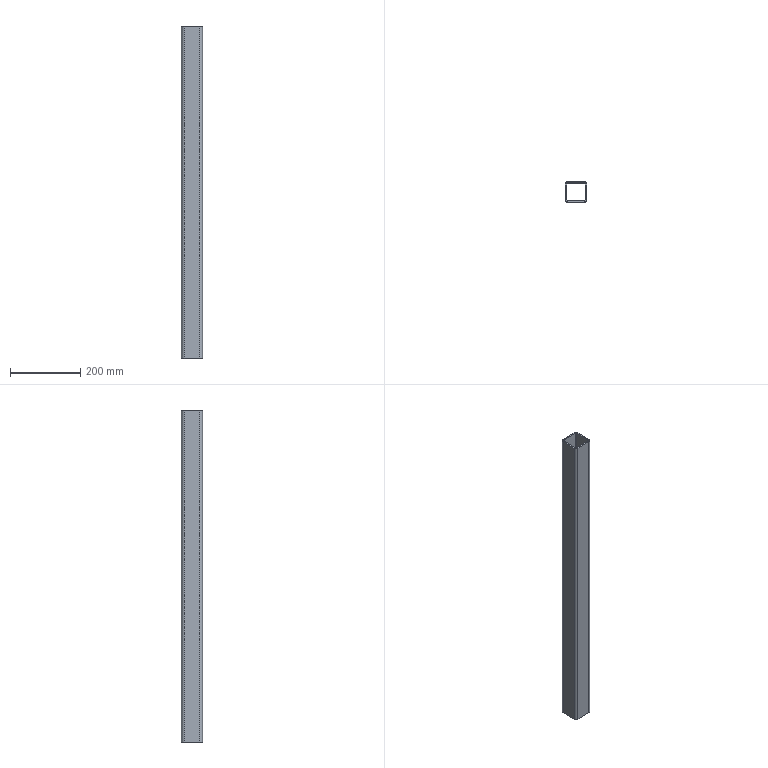Part | SolidWorks | features ICE 1, LibraryFeature 1 | 1 solid | 18 faces | box 60 x 60 x 945 mm | volume 807783 mm3 | plane 10 | cylinder 8 | commonest cylinder face diameters 8 x4 16 x4
STEP:
#1=CARTESIAN_POINT('',(22.,30.,0.));
#2=VERTEX_POINT('',#1);
#3=CARTESIAN_POINT('',(-22.,30.,0.));
#4=VERTEX_POINT('',#3);
#5=CARTESIAN_POINT('',(0.,30.,0.));
#6=DIRECTION('',(-1.,0.,0.));
#7=VECTOR('',#6,1000.);
#8=LINE('',#5,#7);
#9=EDGE_CURVE('',#2,#4,#8,.T.);
#10=ORIENTED_EDGE('',*,*,#9,.T.);
#11=CARTESIAN_POINT('',(-22.,30.,945.));
#12=VERTEX_POINT('',#11);
#13=CARTESIAN_POINT('',(-22.,30.,945.));
#14=DIRECTION('',(0.,0.,-1.));
#15=VECTOR('',#14,1000.);
#16=LINE('',#13,#15);
#17=EDGE_CURVE('',#12,#4,#16,.T.);
#18=ORIENTED_EDGE('',*,*,#17,.F.);
#19=CARTESIAN_POINT('',(22.,30.,945.));
#20=VERTEX_POINT('',#19);
#21=CARTESIAN_POINT('',(0.,30.,945.));
#22=DIRECTION('',(-1.,0.,0.));
#23=VECTOR('',#22,1000.);
#24=LINE('',#21,#23);
#25=EDGE_CURVE('',#20,#12,#24,.T.);
#26=ORIENTED_EDGE('',*,*,#25,.F.);
#27=CARTESIAN_POINT('',(22.,30.,945.));
#28=DIRECTION('',(0.,0.,-1.));
#29=VECTOR('',#28,1000.);
#30=LINE('',#27,#29);
#31=EDGE_CURVE('',#20,#2,#30,.T.);
#32=ORIENTED_EDGE('',*,*,#31,.T.);
#33=EDGE_LOOP('',(#10,#18,#26,#32));
#34=FACE_OUTER_BOUND('',#33,.T.);
#35=CARTESIAN_POINT('',(0.,30.,945.));
#36=DIRECTION('',(0.,-1.,0.));
#37=DIRECTION('',(0.,0.,-1.));
#38=AXIS2_PLACEMENT_3D('',#35,#36,#37);
#39=PLANE('',#38);
#40=ADVANCED_FACE('',(#34),#39,.F.);
#41=CARTESIAN_POINT('',(-30.,22.,0.));
#42=VERTEX_POINT('',#41);
#43=CARTESIAN_POINT('',(-22.,22.,0.));
#44=DIRECTION('',(0.,0.,1.));
#45=DIRECTION('',(1.,0.,0.));
#46=AXIS2_PLACEMENT_3D('',#43,#44,#45);
#47=CIRCLE('',#46,8.);
#48=EDGE_CURVE('',#4,#42,#47,.T.);
#49=ORIENTED_EDGE('',*,*,#48,.T.);
#50=CARTESIAN_POINT('',(-30.,22.,945.));
#51=VERTEX_POINT('',#50);
#52=CARTESIAN_POINT('',(-30.,22.,945.));
#53=DIRECTION('',(0.,0.,-1.));
#54=VECTOR('',#53,1000.);
#55=LINE('',#52,#54);
#56=EDGE_CURVE('',#51,#42,#55,.T.);
#57=ORIENTED_EDGE('',*,*,#56,.F.);
#58=CARTESIAN_POINT('',(-22.,22.,945.));
#59=DIRECTION('',(0.,0.,1.));
#60=DIRECTION('',(1.,0.,0.));
#61=AXIS2_PLACEMENT_3D('',#58,#59,#60);
#62=CIRCLE('',#61,8.);
#63=EDGE_CURVE('',#12,#51,#62,.T.);
#64=ORIENTED_EDGE('',*,*,#63,.F.);
#65=ORIENTED_EDGE('',*,*,#17,.T.);
#66=EDGE_LOOP('',(#49,#57,#64,#65));
#67=FACE_OUTER_BOUND('',#66,.T.);
#68=CARTESIAN_POINT('',(-22.,22.,945.));
#69=DIRECTION('',(0.,0.,-1.));
#70=DIRECTION('',(-1.,0.,0.));
#71=AXIS2_PLACEMENT_3D('',#68,#69,#70);
#72=CYLINDRICAL_SURFACE('',#71,8.);
#73=ADVANCED_FACE('',(#67),#72,.T.);
#74=CARTESIAN_POINT('',(-30.,-22.,0.));
#75=VERTEX_POINT('',#74);
#76=CARTESIAN_POINT('',(-30.,0.,0.));
#77=DIRECTION('',(0.,1.,0.));
#78=VECTOR('',#77,1000.);
#79=LINE('',#76,#78);
#80=EDGE_CURVE('',#75,#42,#79,.T.);
#81=ORIENTED_EDGE('',*,*,#80,.F.);
#82=CARTESIAN_POINT('',(-30.,-22.,945.));
#83=VERTEX_POINT('',#82);
#84=CARTESIAN_POINT('',(-30.,-22.,945.));
#85=DIRECTION('',(0.,0.,-1.));
#86=VECTOR('',#85,1000.);
#87=LINE('',#84,#86);
#88=EDGE_CURVE('',#83,#75,#87,.T.);
#89=ORIENTED_EDGE('',*,*,#88,.F.);
#90=CARTESIAN_POINT('',(-30.,0.,945.));
#91=DIRECTION('',(0.,1.,0.));
#92=VECTOR('',#91,1000.);
#93=LINE('',#90,#92);
#94=EDGE_CURVE('',#83,#51,#93,.T.);
#95=ORIENTED_EDGE('',*,*,#94,.T.);
#96=ORIENTED_EDGE('',*,*,#56,.T.);
#97=EDGE_LOOP('',(#81,#89,#95,#96));
#98=FACE_OUTER_BOUND('',#97,.T.);
#99=CARTESIAN_POINT('',(-30.,0.,945.));
#100=DIRECTION('',(-1.,0.,0.));
#101=DIRECTION('',(0.,0.,1.));
#102=AXIS2_PLACEMENT_3D('',#99,#100,#101);
#103=PLANE('',#102);
#104=ADVANCED_FACE('',(#98),#103,.T.);
#105=CARTESIAN_POINT('',(-22.,-30.,0.));
#106=VERTEX_POINT('',#105);
#107=CARTESIAN_POINT('',(-22.,-22.,0.));
#108=DIRECTION('',(0.,0.,1.));
#109=DIRECTION('',(1.,0.,0.));
#110=AXIS2_PLACEMENT_3D('',#107,#108,#109);
#111=CIRCLE('',#110,8.);
#112=EDGE_CURVE('',#75,#106,#111,.T.);
#113=ORIENTED_EDGE('',*,*,#112,.T.);
#114=CARTESIAN_POINT('',(-22.,-30.,945.));
#115=VERTEX_POINT('',#114);
#116=CARTESIAN_POINT('',(-22.,-30.,945.));
#117=DIRECTION('',(0.,0.,-1.));
#118=VECTOR('',#117,1000.);
#119=LINE('',#116,#118);
#120=EDGE_CURVE('',#115,#106,#119,.T.);
#121=ORIENTED_EDGE('',*,*,#120,.F.);
#122=CARTESIAN_POINT('',(-22.,-22.,945.));
#123=DIRECTION('',(0.,0.,1.));
#124=DIRECTION('',(1.,0.,0.));
#125=AXIS2_PLACEMENT_3D('',#122,#123,#124);
#126=CIRCLE('',#125,8.);
#127=EDGE_CURVE('',#83,#115,#126,.T.);
#128=ORIENTED_EDGE('',*,*,#127,.F.);
#129=ORIENTED_EDGE('',*,*,#88,.T.);
#130=EDGE_LOOP('',(#113,#121,#128,#129));
#131=FACE_OUTER_BOUND('',#130,.T.);
#132=CARTESIAN_POINT('',(-22.,-22.,945.));
#133=DIRECTION('',(0.,0.,-1.));
#134=DIRECTION('',(-1.,0.,0.));
#135=AXIS2_PLACEMENT_3D('',#132,#133,#134);
#136=CYLINDRICAL_SURFACE('',#135,8.);
#137=ADVANCED_FACE('',(#131),#136,.T.);
#138=CARTESIAN_POINT('',(22.,-30.,0.));
#139=VERTEX_POINT('',#138);
#140=CARTESIAN_POINT('',(0.,-30.,0.));
#141=DIRECTION('',(1.,0.,0.));
#142=VECTOR('',#141,1000.);
#143=LINE('',#140,#142);
#144=EDGE_CURVE('',#106,#139,#143,.T.);
#145=ORIENTED_EDGE('',*,*,#144,.T.);
#146=CARTESIAN_POINT('',(22.,-30.,945.));
#147=VERTEX_POINT('',#146);
#148=CARTESIAN_POINT('',(22.,-30.,945.));
#149=DIRECTION('',(0.,0.,-1.));
#150=VECTOR('',#149,1000.);
#151=LINE('',#148,#150);
#152=EDGE_CURVE('',#147,#139,#151,.T.);
#153=ORIENTED_EDGE('',*,*,#152,.F.);
#154=CARTESIAN_POINT('',(0.,-30.,945.));
#155=DIRECTION('',(1.,0.,0.));
#156=VECTOR('',#155,1000.);
#157=LINE('',#154,#156);
#158=EDGE_CURVE('',#115,#147,#157,.T.);
#159=ORIENTED_EDGE('',*,*,#158,.F.);
#160=ORIENTED_EDGE('',*,*,#120,.T.);
#161=EDGE_LOOP('',(#145,#153,#159,#160));
#162=FACE_OUTER_BOUND('',#161,.T.);
#163=CARTESIAN_POINT('',(0.,-30.,945.));
#164=DIRECTION('',(0.,1.,0.));
#165=DIRECTION('',(0.,0.,1.));
#166=AXIS2_PLACEMENT_3D('',#163,#164,#165);
#167=PLANE('',#166);
#168=ADVANCED_FACE('',(#162),#167,.F.);
#169=CARTESIAN_POINT('',(30.,-22.,0.));
#170=VERTEX_POINT('',#169);
#171=CARTESIAN_POINT('',(22.,-22.,0.));
#172=DIRECTION('',(0.,0.,1.));
#173=DIRECTION('',(1.,0.,0.));
#174=AXIS2_PLACEMENT_3D('',#171,#172,#173);
#175=CIRCLE('',#174,8.);
#176=EDGE_CURVE('',#139,#170,#175,.T.);
#177=ORIENTED_EDGE('',*,*,#176,.T.);
#178=CARTESIAN_POINT('',(30.,-22.,945.));
#179=VERTEX_POINT('',#178);
#180=CARTESIAN_POINT('',(30.,-22.,945.));
#181=DIRECTION('',(0.,0.,-1.));
#182=VECTOR('',#181,1000.);
#183=LINE('',#180,#182);
#184=EDGE_CURVE('',#179,#170,#183,.T.);
#185=ORIENTED_EDGE('',*,*,#184,.F.);
#186=CARTESIAN_POINT('',(22.,-22.,945.));
#187=DIRECTION('',(0.,0.,1.));
#188=DIRECTION('',(1.,0.,0.));
#189=AXIS2_PLACEMENT_3D('',#186,#187,#188);
#190=CIRCLE('',#189,8.);
#191=EDGE_CURVE('',#147,#179,#190,.T.);
#192=ORIENTED_EDGE('',*,*,#191,.F.);
#193=ORIENTED_EDGE('',*,*,#152,.T.);
#194=EDGE_LOOP('',(#177,#185,#192,#193));
#195=FACE_OUTER_BOUND('',#194,.T.);
#196=CARTESIAN_POINT('',(22.,-22.,945.));
#197=DIRECTION('',(0.,0.,-1.));
#198=DIRECTION('',(-1.,0.,0.));
#199=AXIS2_PLACEMENT_3D('',#196,#197,#198);
#200=CYLINDRICAL_SURFACE('',#199,8.);
#201=ADVANCED_FACE('',(#195),#200,.T.);
#202=CARTESIAN_POINT('',(30.,22.,0.));
#203=VERTEX_POINT('',#202);
#204=CARTESIAN_POINT('',(30.,0.,0.));
#205=DIRECTION('',(0.,-1.,0.));
#206=VECTOR('',#205,1000.);
#207=LINE('',#204,#206);
#208=EDGE_CURVE('',#203,#170,#207,.T.);
#209=ORIENTED_EDGE('',*,*,#208,.F.);
#210=CARTESIAN_POINT('',(30.,22.,945.));
#211=VERTEX_POINT('',#210);
#212=CARTESIAN_POINT('',(30.,22.,945.));
#213=DIRECTION('',(0.,0.,-1.));
#214=VECTOR('',#213,1000.);
#215=LINE('',#212,#214);
#216=EDGE_CURVE('',#211,#203,#215,.T.);
#217=ORIENTED_EDGE('',*,*,#216,.F.);
#218=CARTESIAN_POINT('',(30.,0.,945.));
#219=DIRECTION('',(0.,-1.,0.));
#220=VECTOR('',#219,1000.);
#221=LINE('',#218,#220);
#222=EDGE_CURVE('',#211,#179,#221,.T.);
#223=ORIENTED_EDGE('',*,*,#222,.T.);
#224=ORIENTED_EDGE('',*,*,#184,.T.);
#225=EDGE_LOOP('',(#209,#217,#223,#224));
#226=FACE_OUTER_BOUND('',#225,.T.);
#227=CARTESIAN_POINT('',(30.,0.,945.));
#228=DIRECTION('',(1.,0.,0.));
#229=DIRECTION('',(0.,0.,-1.));
#230=AXIS2_PLACEMENT_3D('',#227,#228,#229);
#231=PLANE('',#230);
#232=ADVANCED_FACE('',(#226),#231,.T.);
#233=CARTESIAN_POINT('',(-26.,-22.,0.));
#234=VERTEX_POINT('',#233);
#235=CARTESIAN_POINT('',(-22.,-26.,0.));
#236=VERTEX_POINT('',#235);
#237=CARTESIAN_POINT('',(-22.,-22.,0.));
#238=DIRECTION('',(0.,0.,1.));
#239=DIRECTION('',(1.,0.,0.));
#240=AXIS2_PLACEMENT_3D('',#237,#238,#239);
#241=CIRCLE('',#240,4.);
#242=EDGE_CURVE('',#234,#236,#241,.T.);
#243=ORIENTED_EDGE('',*,*,#242,.F.);
#244=CARTESIAN_POINT('',(-26.,-22.,945.));
#245=VERTEX_POINT('',#244);
#246=CARTESIAN_POINT('',(-26.,-22.,945.));
#247=DIRECTION('',(0.,0.,-1.));
#248=VECTOR('',#247,1000.);
#249=LINE('',#246,#248);
#250=EDGE_CURVE('',#245,#234,#249,.T.);
#251=ORIENTED_EDGE('',*,*,#250,.F.);
#252=CARTESIAN_POINT('',(-22.,-26.,945.));
#253=VERTEX_POINT('',#252);
#254=CARTESIAN_POINT('',(-22.,-22.,945.));
#255=DIRECTION('',(0.,0.,1.));
#256=DIRECTION('',(1.,0.,0.));
#257=AXIS2_PLACEMENT_3D('',#254,#255,#256);
#258=CIRCLE('',#257,4.);
#259=EDGE_CURVE('',#245,#253,#258,.T.);
#260=ORIENTED_EDGE('',*,*,#259,.T.);
#261=CARTESIAN_POINT('',(-22.,-26.,945.));
#262=DIRECTION('',(0.,0.,-1.));
#263=VECTOR('',#262,1000.);
#264=LINE('',#261,#263);
#265=EDGE_CURVE('',#253,#236,#264,.T.);
#266=ORIENTED_EDGE('',*,*,#265,.T.);
#267=EDGE_LOOP('',(#243,#251,#260,#266));
#268=FACE_OUTER_BOUND('',#267,.T.);
#269=CARTESIAN_POINT('',(-22.,-22.,945.));
#270=DIRECTION('',(0.,0.,-1.));
#271=DIRECTION('',(-1.,0.,0.));
#272=AXIS2_PLACEMENT_3D('',#269,#270,#271);
#273=CYLINDRICAL_SURFACE('',#272,4.);
#274=ADVANCED_FACE('',(#268),#273,.F.);
#275=CARTESIAN_POINT('',(-26.,22.,0.));
#276=VERTEX_POINT('',#275);
#277=CARTESIAN_POINT('',(-26.,0.,0.));
#278=DIRECTION('',(0.,1.,0.));
#279=VECTOR('',#278,1000.);
#280=LINE('',#277,#279);
#281=EDGE_CURVE('',#234,#276,#280,.T.);
#282=ORIENTED_EDGE('',*,*,#281,.T.);
#283=CARTESIAN_POINT('',(-26.,22.,945.));
#284=VERTEX_POINT('',#283);
#285=CARTESIAN_POINT('',(-26.,22.,945.));
#286=DIRECTION('',(0.,0.,-1.));
#287=VECTOR('',#286,1000.);
#288=LINE('',#285,#287);
#289=EDGE_CURVE('',#284,#276,#288,.T.);
#290=ORIENTED_EDGE('',*,*,#289,.F.);
#291=CARTESIAN_POINT('',(-26.,0.,945.));
#292=DIRECTION('',(0.,1.,0.));
#293=VECTOR('',#292,1000.);
#294=LINE('',#291,#293);
#295=EDGE_CURVE('',#245,#284,#294,.T.);
#296=ORIENTED_EDGE('',*,*,#295,.F.);
#297=ORIENTED_EDGE('',*,*,#250,.T.);
#298=EDGE_LOOP('',(#282,#290,#296,#297));
#299=FACE_OUTER_BOUND('',#298,.T.);
#300=CARTESIAN_POINT('',(-26.,0.,945.));
#301=DIRECTION('',(-1.,0.,0.));
#302=DIRECTION('',(0.,0.,1.));
#303=AXIS2_PLACEMENT_3D('',#300,#301,#302);
#304=PLANE('',#303);
#305=ADVANCED_FACE('',(#299),#304,.F.);
#306=CARTESIAN_POINT('',(-22.,26.,0.));
#307=VERTEX_POINT('',#306);
#308=CARTESIAN_POINT('',(-22.,22.,0.));
#309=DIRECTION('',(0.,0.,1.));
#310=DIRECTION('',(1.,0.,0.));
#311=AXIS2_PLACEMENT_3D('',#308,#309,#310);
#312=CIRCLE('',#311,4.);
#313=EDGE_CURVE('',#307,#276,#312,.T.);
#314=ORIENTED_EDGE('',*,*,#313,.F.);
#315=CARTESIAN_POINT('',(-22.,26.,945.));
#316=VERTEX_POINT('',#315);
#317=CARTESIAN_POINT('',(-22.,26.,945.));
#318=DIRECTION('',(0.,0.,-1.));
#319=VECTOR('',#318,1000.);
#320=LINE('',#317,#319);
#321=EDGE_CURVE('',#316,#307,#320,.T.);
#322=ORIENTED_EDGE('',*,*,#321,.F.);
#323=CARTESIAN_POINT('',(-22.,22.,945.));
#324=DIRECTION('',(0.,0.,1.));
#325=DIRECTION('',(1.,0.,0.));
#326=AXIS2_PLACEMENT_3D('',#323,#324,#325);
#327=CIRCLE('',#326,4.);
#328=EDGE_CURVE('',#316,#284,#327,.T.);
#329=ORIENTED_EDGE('',*,*,#328,.T.);
#330=ORIENTED_EDGE('',*,*,#289,.T.);
#331=EDGE_LOOP('',(#314,#322,#329,#330));
#332=FACE_OUTER_BOUND('',#331,.T.);
#333=CARTESIAN_POINT('',(-22.,22.,945.));
#334=DIRECTION('',(0.,0.,-1.));
#335=DIRECTION('',(-1.,0.,0.));
#336=AXIS2_PLACEMENT_3D('',#333,#334,#335);
#337=CYLINDRICAL_SURFACE('',#336,4.);
#338=ADVANCED_FACE('',(#332),#337,.F.);
#339=CARTESIAN_POINT('',(22.,26.,0.));
#340=VERTEX_POINT('',#339);
#341=CARTESIAN_POINT('',(0.,26.,0.));
#342=DIRECTION('',(-1.,0.,0.));
#343=VECTOR('',#342,1000.);
#344=LINE('',#341,#343);
#345=EDGE_CURVE('',#340,#307,#344,.T.);
#346=ORIENTED_EDGE('',*,*,#345,.F.);
#347=CARTESIAN_POINT('',(22.,26.,945.));
#348=VERTEX_POINT('',#347);
#349=CARTESIAN_POINT('',(22.,26.,945.));
#350=DIRECTION('',(0.,0.,-1.));
#351=VECTOR('',#350,1000.);
#352=LINE('',#349,#351);
#353=EDGE_CURVE('',#348,#340,#352,.T.);
#354=ORIENTED_EDGE('',*,*,#353,.F.);
#355=CARTESIAN_POINT('',(0.,26.,945.));
#356=DIRECTION('',(-1.,0.,0.));
#357=VECTOR('',#356,1000.);
#358=LINE('',#355,#357);
#359=EDGE_CURVE('',#348,#316,#358,.T.);
#360=ORIENTED_EDGE('',*,*,#359,.T.);
#361=ORIENTED_EDGE('',*,*,#321,.T.);
#362=EDGE_LOOP('',(#346,#354,#360,#361));
#363=FACE_OUTER_BOUND('',#362,.T.);
#364=CARTESIAN_POINT('',(0.,26.,945.));
#365=DIRECTION('',(0.,-1.,0.));
#366=DIRECTION('',(0.,0.,-1.));
#367=AXIS2_PLACEMENT_3D('',#364,#365,#366);
#368=PLANE('',#367);
#369=ADVANCED_FACE('',(#363),#368,.T.);
#370=CARTESIAN_POINT('',(26.,22.,0.));
#371=VERTEX_POINT('',#370);
#372=CARTESIAN_POINT('',(22.,22.,0.));
#373=DIRECTION('',(0.,0.,1.));
#374=DIRECTION('',(1.,0.,0.));
#375=AXIS2_PLACEMENT_3D('',#372,#373,#374);
#376=CIRCLE('',#375,4.);
#377=EDGE_CURVE('',#371,#340,#376,.T.);
#378=ORIENTED_EDGE('',*,*,#377,.F.);
#379=CARTESIAN_POINT('',(26.,22.,945.));
#380=VERTEX_POINT('',#379);
#381=CARTESIAN_POINT('',(26.,22.,945.));
#382=DIRECTION('',(0.,0.,-1.));
#383=VECTOR('',#382,1000.);
#384=LINE('',#381,#383);
#385=EDGE_CURVE('',#380,#371,#384,.T.);
#386=ORIENTED_EDGE('',*,*,#385,.F.);
#387=CARTESIAN_POINT('',(22.,22.,945.));
#388=DIRECTION('',(0.,0.,1.));
#389=DIRECTION('',(1.,0.,0.));
#390=AXIS2_PLACEMENT_3D('',#387,#388,#389);
#391=CIRCLE('',#390,4.);
#392=EDGE_CURVE('',#380,#348,#391,.T.);
#393=ORIENTED_EDGE('',*,*,#392,.T.);
#394=ORIENTED_EDGE('',*,*,#353,.T.);
#395=EDGE_LOOP('',(#378,#386,#393,#394));
#396=FACE_OUTER_BOUND('',#395,.T.);
#397=CARTESIAN_POINT('',(22.,22.,945.));
#398=DIRECTION('',(0.,0.,-1.));
#399=DIRECTION('',(-1.,0.,0.));
#400=AXIS2_PLACEMENT_3D('',#397,#398,#399);
#401=CYLINDRICAL_SURFACE('',#400,4.);
#402=ADVANCED_FACE('',(#396),#401,.F.);
#403=CARTESIAN_POINT('',(26.,-22.,0.));
#404=VERTEX_POINT('',#403);
#405=CARTESIAN_POINT('',(26.,0.,0.));
#406=DIRECTION('',(0.,-1.,0.));
#407=VECTOR('',#406,1000.);
#408=LINE('',#405,#407);
#409=EDGE_CURVE('',#371,#404,#408,.T.);
#410=ORIENTED_EDGE('',*,*,#409,.T.);
#411=CARTESIAN_POINT('',(26.,-22.,945.));
#412=VERTEX_POINT('',#411);
#413=CARTESIAN_POINT('',(26.,-22.,945.));
#414=DIRECTION('',(0.,0.,-1.));
#415=VECTOR('',#414,1000.);
#416=LINE('',#413,#415);
#417=EDGE_CURVE('',#412,#404,#416,.T.);
#418=ORIENTED_EDGE('',*,*,#417,.F.);
#419=CARTESIAN_POINT('',(26.,0.,945.));
#420=DIRECTION('',(0.,-1.,0.));
#421=VECTOR('',#420,1000.);
#422=LINE('',#419,#421);
#423=EDGE_CURVE('',#380,#412,#422,.T.);
#424=ORIENTED_EDGE('',*,*,#423,.F.);
#425=ORIENTED_EDGE('',*,*,#385,.T.);
#426=EDGE_LOOP('',(#410,#418,#424,#425));
#427=FACE_OUTER_BOUND('',#426,.T.);
#428=CARTESIAN_POINT('',(26.,0.,945.));
#429=DIRECTION('',(1.,0.,0.));
#430=DIRECTION('',(0.,0.,-1.));
#431=AXIS2_PLACEMENT_3D('',#428,#429,#430);
#432=PLANE('',#431);
#433=ADVANCED_FACE('',(#427),#432,.F.);
#434=CARTESIAN_POINT('',(22.,-26.,0.));
#435=VERTEX_POINT('',#434);
#436=CARTESIAN_POINT('',(22.,-22.,0.));
#437=DIRECTION('',(0.,0.,1.));
#438=DIRECTION('',(1.,0.,0.));
#439=AXIS2_PLACEMENT_3D('',#436,#437,#438);
#440=CIRCLE('',#439,4.);
#441=EDGE_CURVE('',#435,#404,#440,.T.);
#442=ORIENTED_EDGE('',*,*,#441,.F.);
#443=CARTESIAN_POINT('',(22.,-26.,945.));
#444=VERTEX_POINT('',#443);
#445=CARTESIAN_POINT('',(22.,-26.,945.));
#446=DIRECTION('',(0.,0.,-1.));
#447=VECTOR('',#446,1000.);
#448=LINE('',#445,#447);
#449=EDGE_CURVE('',#444,#435,#448,.T.);
#450=ORIENTED_EDGE('',*,*,#449,.F.);
#451=CARTESIAN_POINT('',(22.,-22.,945.));
#452=DIRECTION('',(0.,0.,1.));
#453=DIRECTION('',(1.,0.,0.));
#454=AXIS2_PLACEMENT_3D('',#451,#452,#453);
#455=CIRCLE('',#454,4.);
#456=EDGE_CURVE('',#444,#412,#455,.T.);
#457=ORIENTED_EDGE('',*,*,#456,.T.);
#458=ORIENTED_EDGE('',*,*,#417,.T.);
#459=EDGE_LOOP('',(#442,#450,#457,#458));
#460=FACE_OUTER_BOUND('',#459,.T.);
#461=CARTESIAN_POINT('',(22.,-22.,945.));
#462=DIRECTION('',(0.,0.,-1.));
#463=DIRECTION('',(-1.,0.,0.));
#464=AXIS2_PLACEMENT_3D('',#461,#462,#463);
#465=CYLINDRICAL_SURFACE('',#464,4.);
#466=ADVANCED_FACE('',(#460),#465,.F.);
#467=CARTESIAN_POINT('',(0.,-26.,0.));
#468=DIRECTION('',(1.,0.,0.));
#469=VECTOR('',#468,1000.);
#470=LINE('',#467,#469);
#471=EDGE_CURVE('',#236,#435,#470,.T.);
#472=ORIENTED_EDGE('',*,*,#471,.F.);
#473=ORIENTED_EDGE('',*,*,#265,.F.);
#474=CARTESIAN_POINT('',(0.,-26.,945.));
#475=DIRECTION('',(1.,0.,0.));
#476=VECTOR('',#475,1000.);
#477=LINE('',#474,#476);
#478=EDGE_CURVE('',#253,#444,#477,.T.);
#479=ORIENTED_EDGE('',*,*,#478,.T.);
#480=ORIENTED_EDGE('',*,*,#449,.T.);
#481=EDGE_LOOP('',(#472,#473,#479,#480));
#482=FACE_OUTER_BOUND('',#481,.T.);
#483=CARTESIAN_POINT('',(0.,-26.,945.));
#484=DIRECTION('',(0.,1.,0.));
#485=DIRECTION('',(0.,0.,1.));
#486=AXIS2_PLACEMENT_3D('',#483,#484,#485);
#487=PLANE('',#486);
#488=ADVANCED_FACE('',(#482),#487,.T.);
#489=CARTESIAN_POINT('',(22.,22.,0.));
#490=DIRECTION('',(0.,0.,1.));
#491=DIRECTION('',(1.,0.,0.));
#492=AXIS2_PLACEMENT_3D('',#489,#490,#491);
#493=CIRCLE('',#492,8.);
#494=EDGE_CURVE('',#203,#2,#493,.T.);
#495=ORIENTED_EDGE('',*,*,#494,.T.);
#496=ORIENTED_EDGE('',*,*,#31,.F.);
#497=CARTESIAN_POINT('',(22.,22.,945.));
#498=DIRECTION('',(0.,0.,1.));
#499=DIRECTION('',(1.,0.,0.));
#500=AXIS2_PLACEMENT_3D('',#497,#498,#499);
#501=CIRCLE('',#500,8.);
#502=EDGE_CURVE('',#211,#20,#501,.T.);
#503=ORIENTED_EDGE('',*,*,#502,.F.);
#504=ORIENTED_EDGE('',*,*,#216,.T.);
#505=EDGE_LOOP('',(#495,#496,#503,#504));
#506=FACE_OUTER_BOUND('',#505,.T.);
#507=CARTESIAN_POINT('',(22.,22.,945.));
#508=DIRECTION('',(0.,0.,-1.));
#509=DIRECTION('',(-1.,0.,0.));
#510=AXIS2_PLACEMENT_3D('',#507,#508,#509);
#511=CYLINDRICAL_SURFACE('',#510,8.);
#512=ADVANCED_FACE('',(#506),#511,.T.);
#513=ORIENTED_EDGE('',*,*,#259,.F.);
#514=ORIENTED_EDGE('',*,*,#295,.T.);
#515=ORIENTED_EDGE('',*,*,#328,.F.);
#516=ORIENTED_EDGE('',*,*,#359,.F.);
#517=ORIENTED_EDGE('',*,*,#392,.F.);
#518=ORIENTED_EDGE('',*,*,#423,.T.);
#519=ORIENTED_EDGE('',*,*,#456,.F.);
#520=ORIENTED_EDGE('',*,*,#478,.F.);
#521=EDGE_LOOP('',(#513,#514,#515,#516,#517,#518,#519,#520));
#522=FACE_BOUND('',#521,.T.);
#523=ORIENTED_EDGE('',*,*,#25,.T.);
#524=ORIENTED_EDGE('',*,*,#63,.T.);
#525=ORIENTED_EDGE('',*,*,#94,.F.);
#526=ORIENTED_EDGE('',*,*,#127,.T.);
#527=ORIENTED_EDGE('',*,*,#158,.T.);
#528=ORIENTED_EDGE('',*,*,#191,.T.);
#529=ORIENTED_EDGE('',*,*,#222,.F.);
#530=ORIENTED_EDGE('',*,*,#502,.T.);
#531=EDGE_LOOP('',(#523,#524,#525,#526,#527,#528,#529,#530));
#532=FACE_OUTER_BOUND('',#531,.T.);
#533=CARTESIAN_POINT('',(0.,0.,945.));
#534=DIRECTION('',(0.,0.,1.));
#535=DIRECTION('',(1.,0.,0.));
#536=AXIS2_PLACEMENT_3D('',#533,#534,#535);
#537=PLANE('',#536);
#538=ADVANCED_FACE('',(#522,#532),#537,.T.);
#539=ORIENTED_EDGE('',*,*,#242,.T.);
#540=ORIENTED_EDGE('',*,*,#471,.T.);
#541=ORIENTED_EDGE('',*,*,#441,.T.);
#542=ORIENTED_EDGE('',*,*,#409,.F.);
#543=ORIENTED_EDGE('',*,*,#377,.T.);
#544=ORIENTED_EDGE('',*,*,#345,.T.);
#545=ORIENTED_EDGE('',*,*,#313,.T.);
#546=ORIENTED_EDGE('',*,*,#281,.F.);
#547=EDGE_LOOP('',(#539,#540,#541,#542,#543,#544,#545,#546));
#548=FACE_BOUND('',#547,.T.);
#549=ORIENTED_EDGE('',*,*,#9,.F.);
#550=ORIENTED_EDGE('',*,*,#494,.F.);
#551=ORIENTED_EDGE('',*,*,#208,.T.);
#552=ORIENTED_EDGE('',*,*,#176,.F.);
#553=ORIENTED_EDGE('',*,*,#144,.F.);
#554=ORIENTED_EDGE('',*,*,#112,.F.);
#555=ORIENTED_EDGE('',*,*,#80,.T.);
#556=ORIENTED_EDGE('',*,*,#48,.F.);
#557=EDGE_LOOP('',(#549,#550,#551,#552,#553,#554,#555,#556));
#558=FACE_OUTER_BOUND('',#557,.T.);
#559=CARTESIAN_POINT('',(0.,0.,0.));
#560=DIRECTION('',(0.,0.,1.));
#561=DIRECTION('',(1.,0.,0.));
#562=AXIS2_PLACEMENT_3D('',#559,#560,#561);
#563=PLANE('',#562);
#564=ADVANCED_FACE('',(#548,#558),#563,.F.);
#565=CLOSED_SHELL('',(#40,#73,#104,#137,#168,#201,#232,#274,#305,#338,#369,#402,#433,#466,#488,#512,#538,#564));
#566=MANIFOLD_SOLID_BREP('',#565);
#567=CARTESIAN_POINT('',(0.,0.,0.));
#568=DIRECTION('',(0.,0.,1.));
#569=DIRECTION('',(1.,0.,0.));
#570=AXIS2_PLACEMENT_3D('',#567,#568,#569);
#571=(LENGTH_UNIT()NAMED_UNIT(*)SI_UNIT(.MILLI.,.METRE.));
#572=UNCERTAINTY_MEASURE_WITH_UNIT(LENGTH_MEASURE(0.00001),#571,'','');
#573=(NAMED_UNIT(*)PLANE_ANGLE_UNIT()SI_UNIT($,.RADIAN.));
#574=(NAMED_UNIT(*)SI_UNIT($,.STERADIAN.)SOLID_ANGLE_UNIT());
#575=(GEOMETRIC_REPRESENTATION_CONTEXT(3)GLOBAL_UNCERTAINTY_ASSIGNED_CONTEXT((#572))GLOBAL_UNIT_ASSIGNED_CONTEXT((#571,#573,#574))REPRESENTATION_CONTEXT('',''));
#576=ADVANCED_BREP_SHAPE_REPRESENTATION('',(#566,#570),#575);